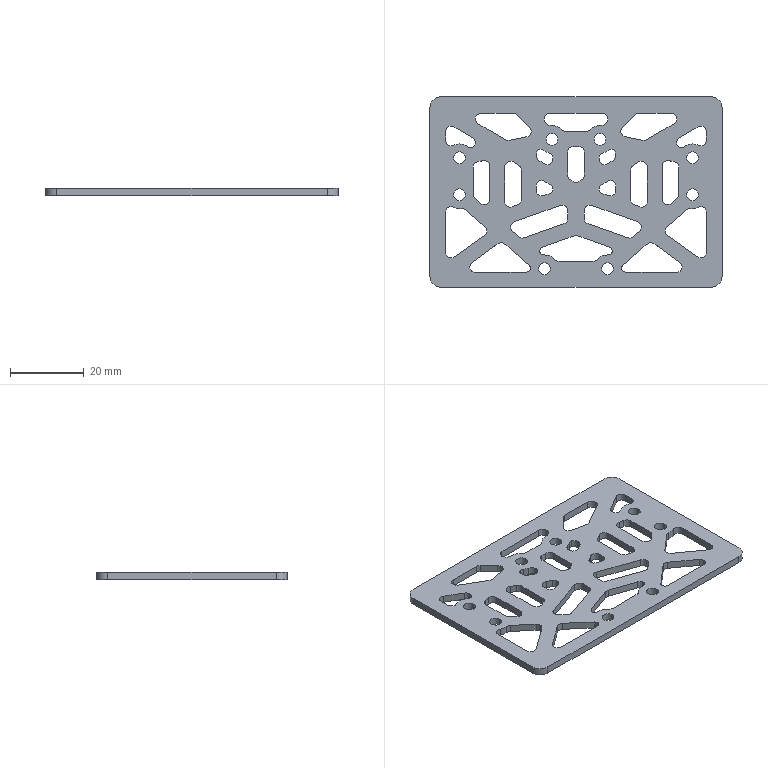Part | SolidWorks | features Fillet 5, ICE 3, Extrusion 1 | 1 solid | 215 faces | box 79 x 51.5 x 2 mm | volume 5613 mm3 | cylinder 137 | plane 78 | commonest cylinder face diameters 3 x98 3.2 x16 7.5 x10 2 x9 6 x4